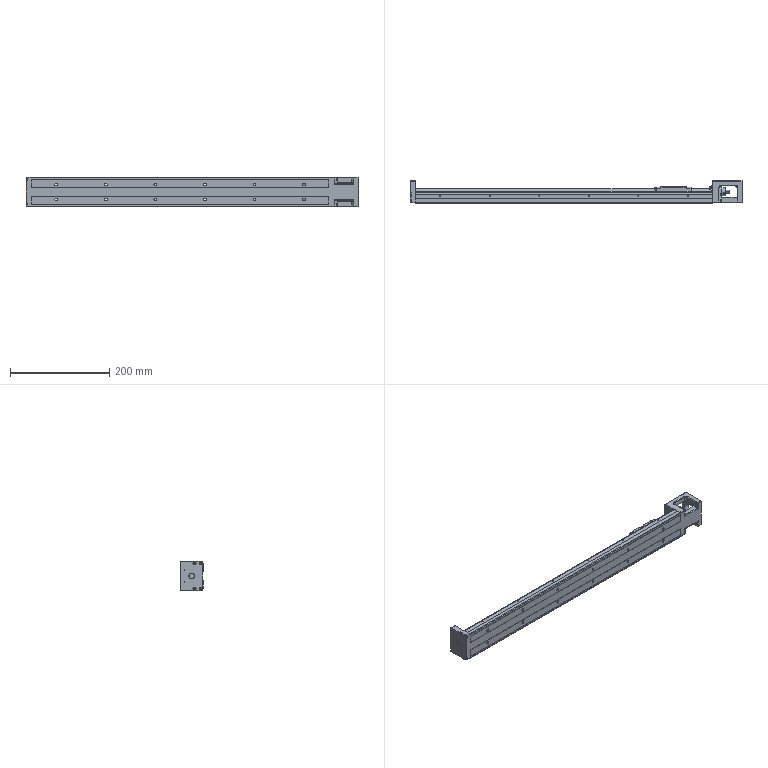Part | NX | features BREP 3 | 1 solid | 628 faces | box 670 x 44.5 x 60 mm | volume 537921 mm3 | plane 339 | cylinder 234 | cone 26 | torus 24 | sphere 5 | commonest cylinder face diameters 5.5 x40 3 x30 2.15 x28 9.5 x24 6 x22 3.3 x18